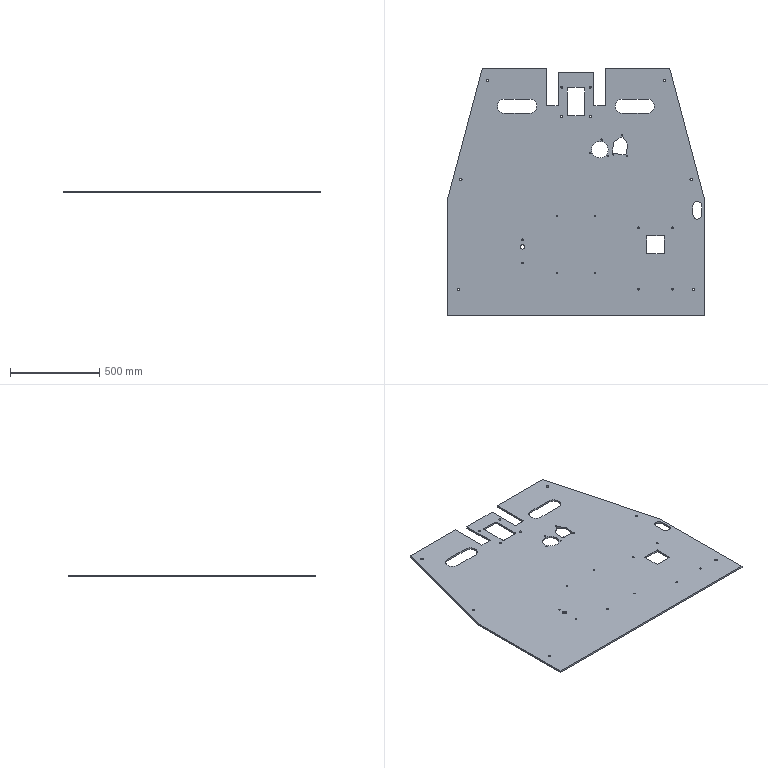Part | SolidWorks | features ICE 21, LPattern 10, Extrusion 1, Fillet 1 | 1 solid | 103 faces | box 1440 x 1385 x 10 mm | volume 17401314 mm3 | cylinder 68 | plane 35 | commonest cylinder face diameters 8 x14 10 x12 14 x12 12 x8 6 x6 80 x6